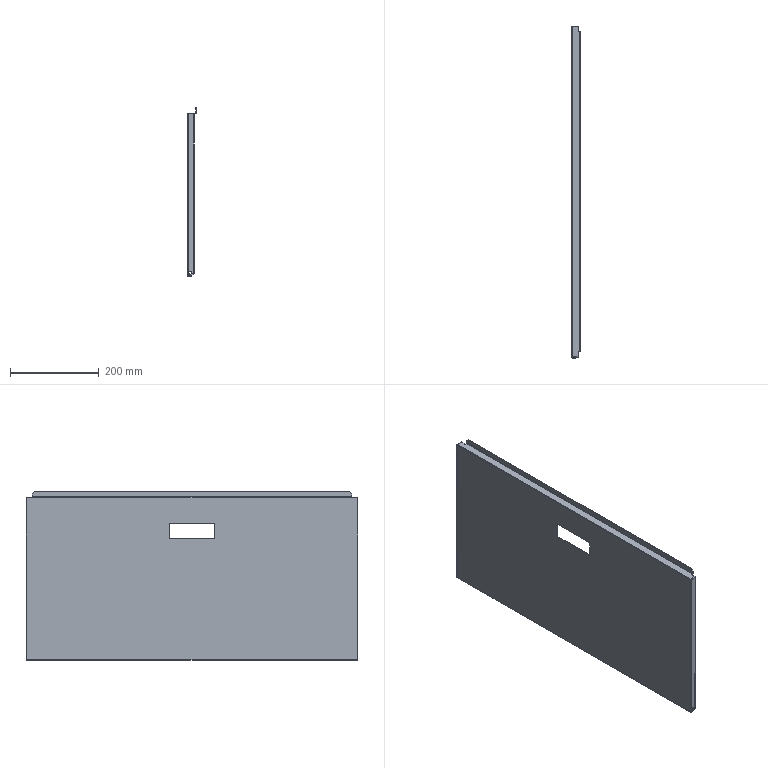Part | SolidWorks | features EdgeFlange 6, ICE 5, Chamfer 1, FlatPattern 1, SMBaseFlange 1, SheetMetal 1 | 1 solid | 96 faces | box 20.237 x 747 x 379.5 mm | volume 479415 mm3 | plane 76 | cylinder 20 | commonest cylinder face diameters 0.6 x6 3.6 x6 7 x4 1.473 x2 4.473 x2